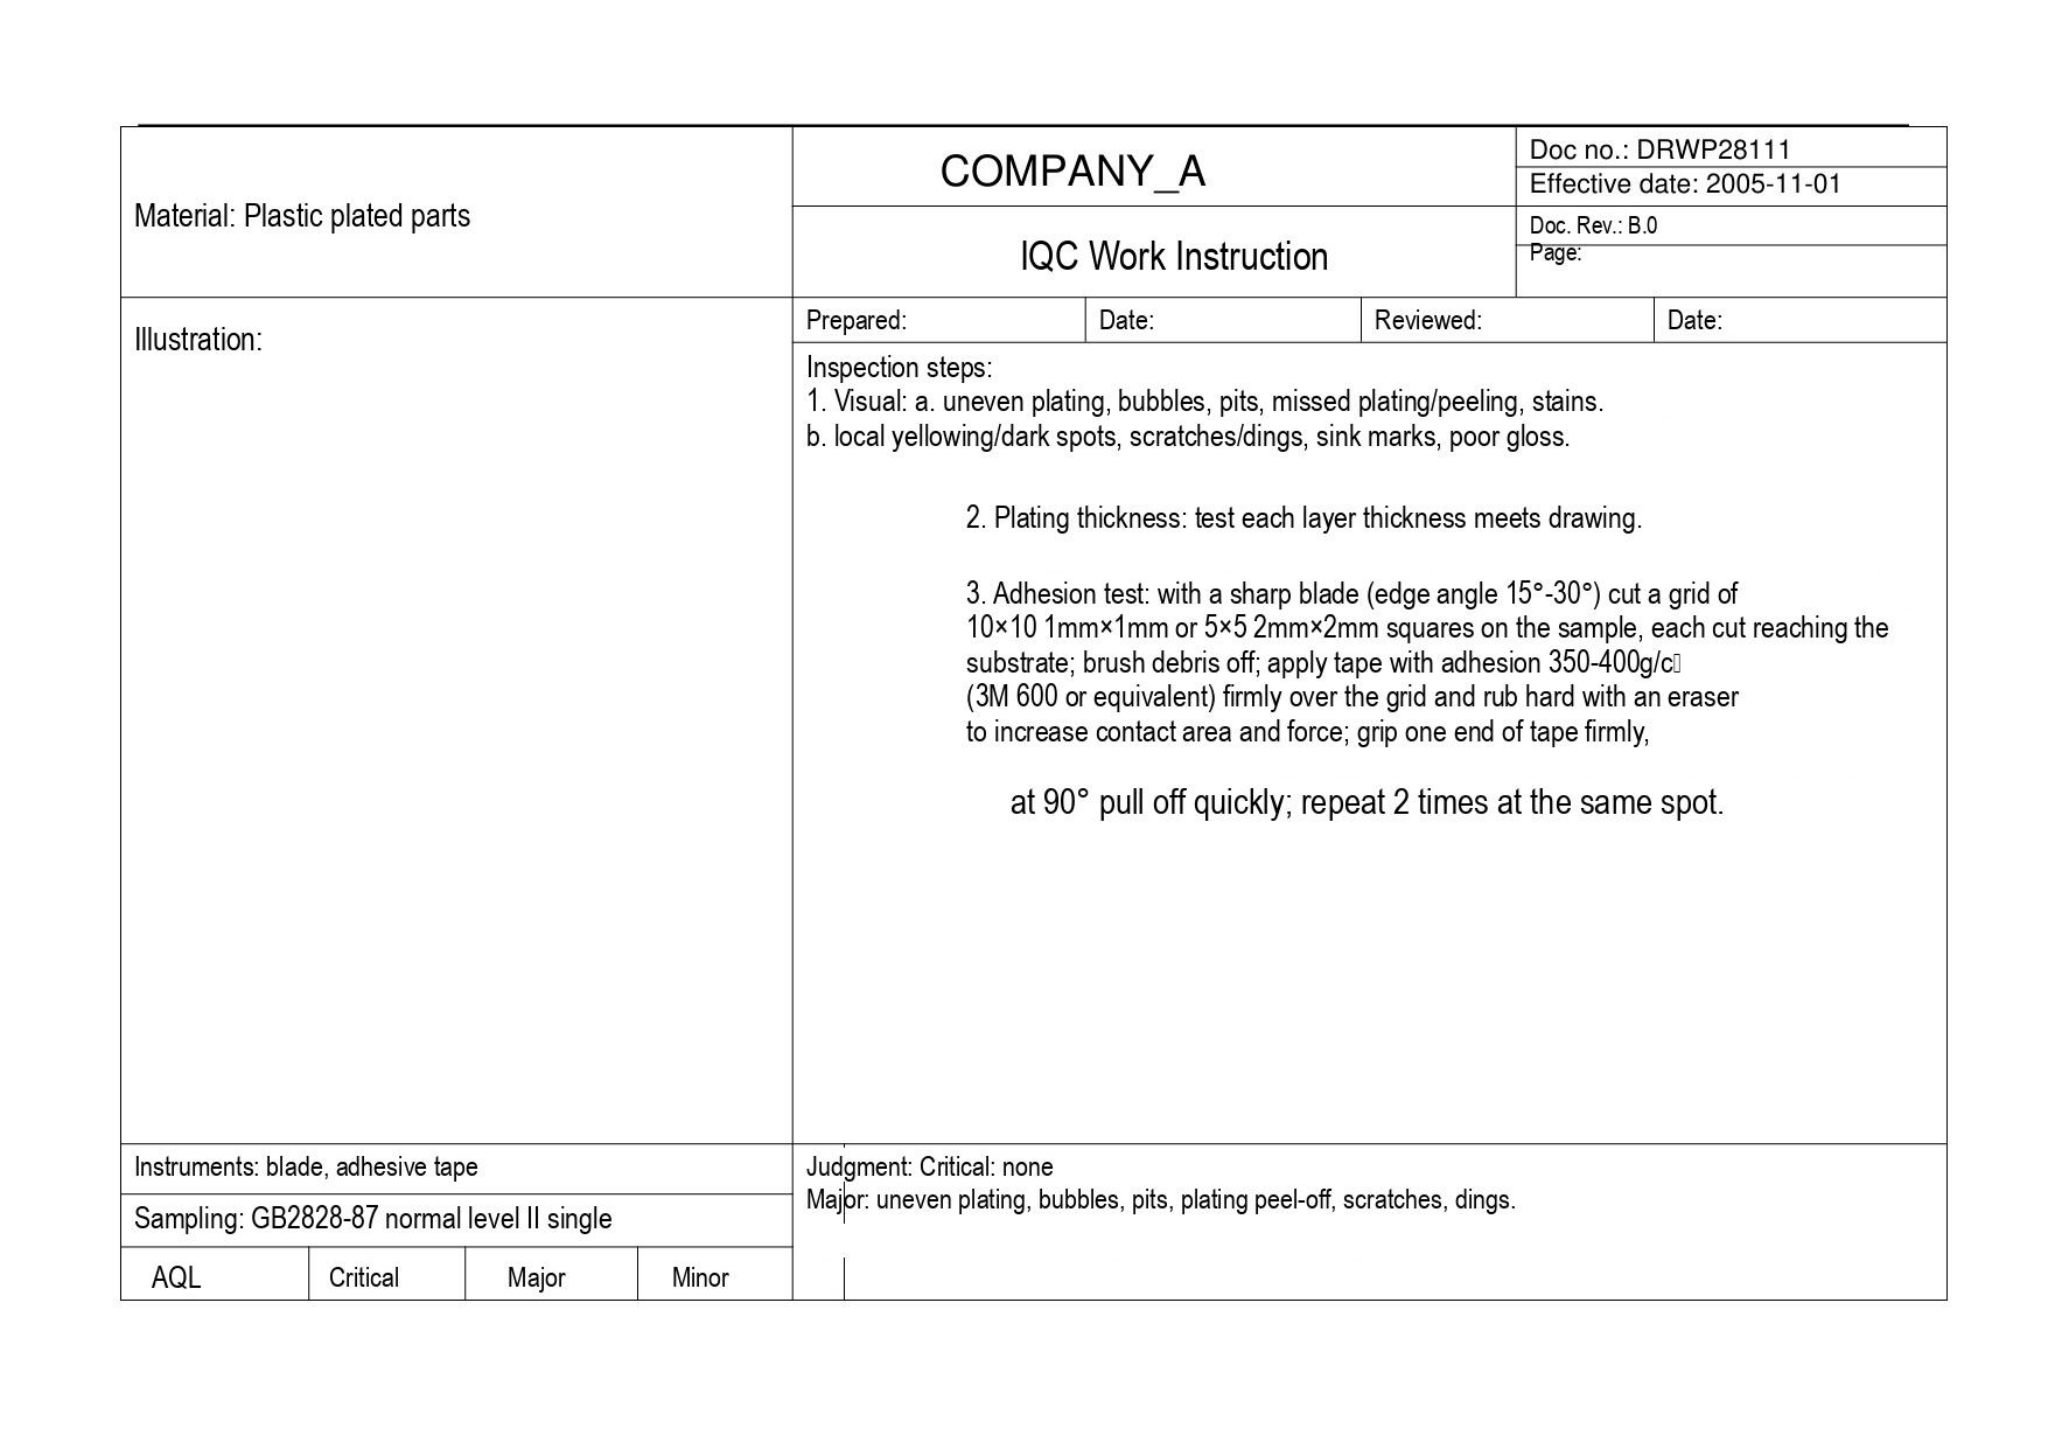| Material: Plastic plated parts | COMPANY_A | Doc no.: DRWP28111 |
|---|---|---|
| | | Effective date: 2005-11-01 |
| | IQC Work Instruction | Doc. Rev.: B.0 |
| | | Page: |

| Prepared: | Date: | Reviewed: | Date: |
|---|---|---|---|

Illustration:

Inspection steps:
1. Visual: a. uneven plating, bubbles, pits, missed plating/peeling, stains.
b. local yellowing/dark spots, scratches/dings, sink marks, poor gloss.

2. Plating thickness: test each layer thickness meets drawing.

3. Adhesion test: with a sharp blade (edge angle 15°-30°) cut a grid of 10×10 1mm×1mm or 5×5 2mm×2mm squares on the sample, each cut reaching the substrate; brush debris off; apply tape with adhesion 350-400g/c
(3M 600 or equivalent) firmly over the grid and rub hard with an eraser to increase contact area and force; grip one end of tape firmly,

at 90° pull off quickly; repeat 2 times at the same spot.

Instruments: blade, adhesive tape

Sampling: GB2828-87 normal level II single

| AQL | Critical | Major | Minor |
|---|---|---|---|

Judgment: Critical: none
Major: uneven plating, bubbles, pits, plating peel-off, scratches, dings.
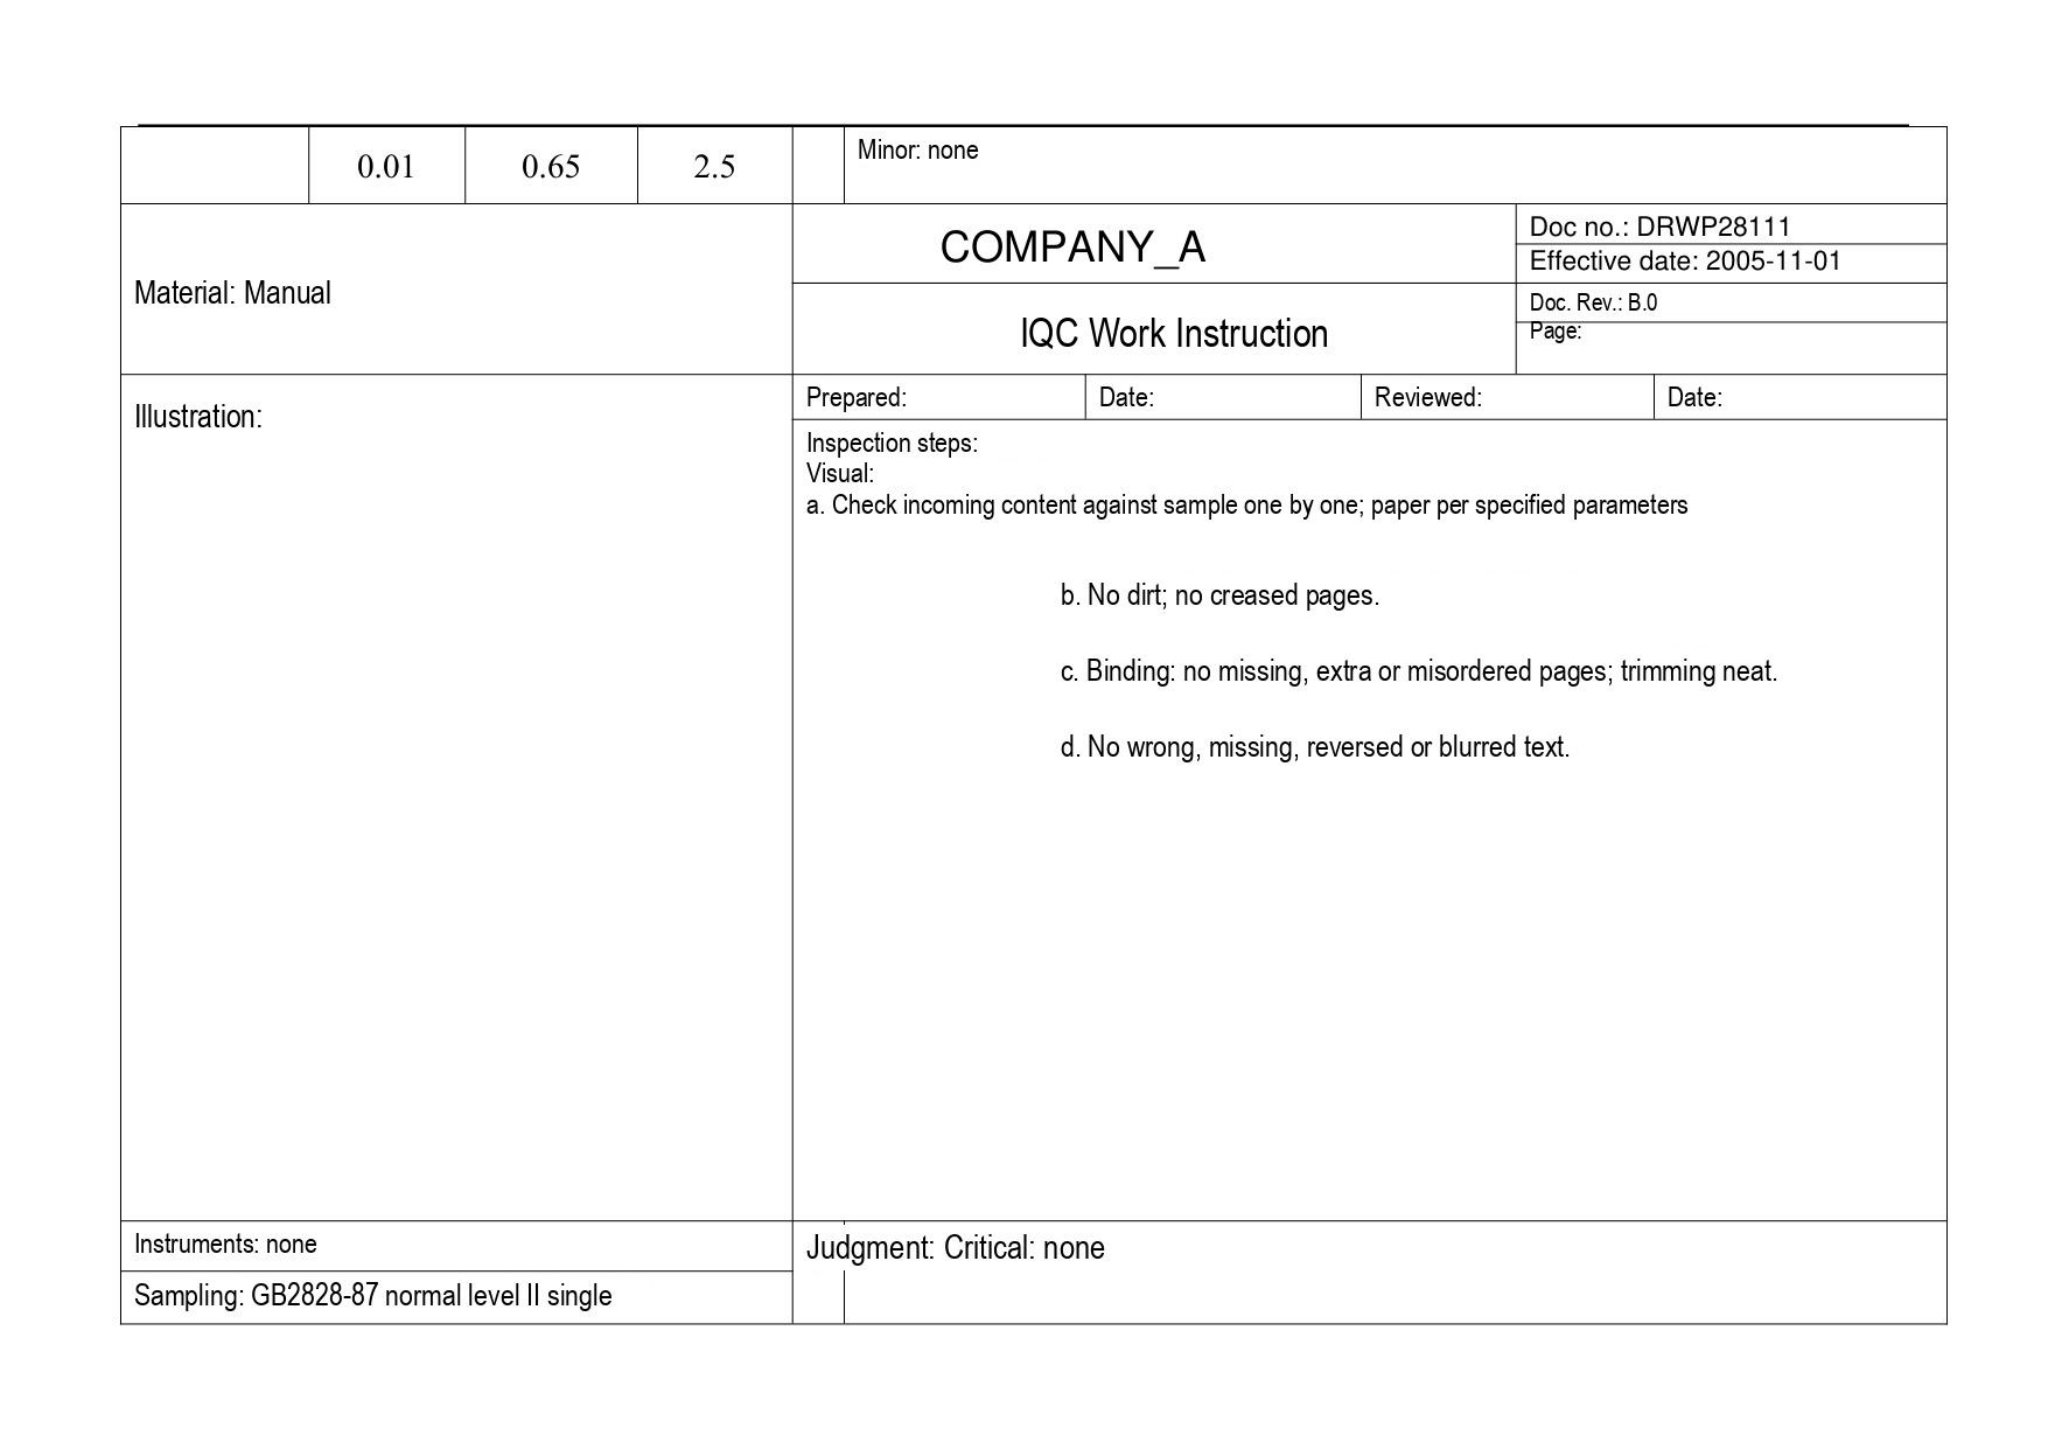| | 0.01 | 0.65 | 2.5 | | Minor: none |
|---|---|---|---|---|---|

Material: Manual

COMPANY_A

IQC Work Instruction

| Doc no.: DRWP28111 |
|---|
| Effective date: 2005-11-01 |
| Doc. Rev.: B.0 |
| Page: |

Illustration:

| Prepared: | Date: | Reviewed: | Date: |
|---|---|---|---|

Inspection steps:
Visual:
a. Check incoming content against sample one by one; paper per specified parameters

b. No dirt; no creased pages.

c. Binding: no missing, extra or misordered pages; trimming neat.

d. No wrong, missing, reversed or blurred text.

Instruments: none

Sampling: GB2828-87 normal level II single

Judgment: Critical: none
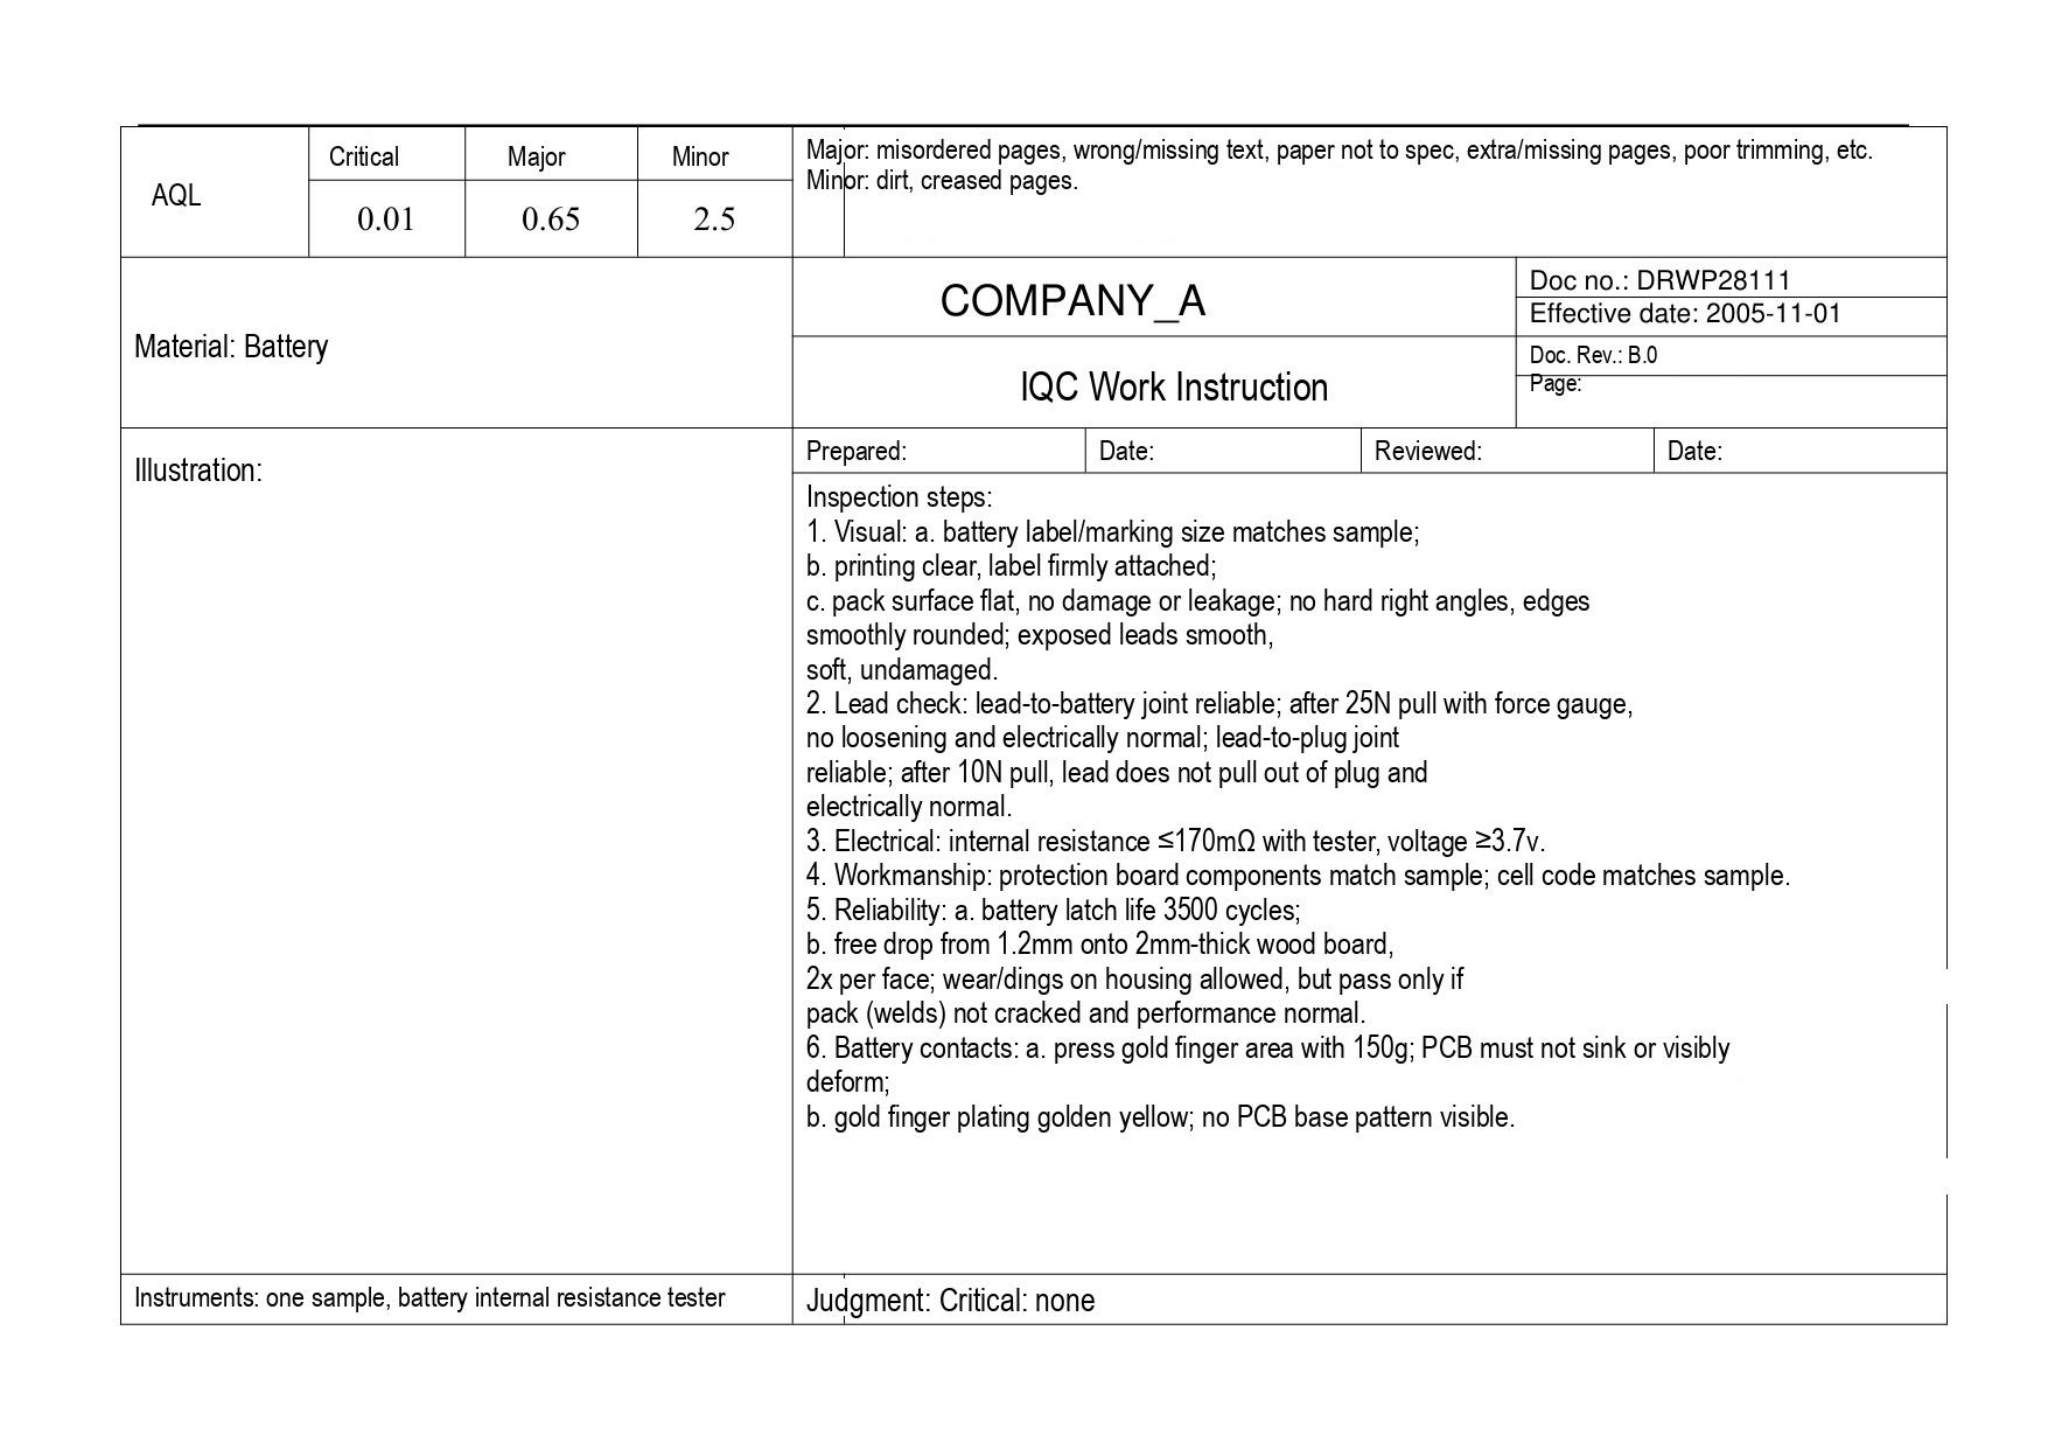| AQL | Critical | Major | Minor |
|---|---|---|---|
| | 0.01 | 0.65 | 2.5 |

Major: misordered pages, wrong/missing text, paper not to spec, extra/missing pages, poor trimming, etc.
Minor: dirt, creased pages.

| Material: Battery | COMPANY_A | Doc no.: DRWP28111 |
|---|---|---|
| | | Effective date: 2005-11-01 |
| | IQC Work Instruction | Doc. Rev.: B.0 |
| | | Page: |

| Prepared: | Date: | Reviewed: | Date: |
|---|---|---|---|

Illustration:

Inspection steps:
1. Visual: a. battery label/marking size matches sample;
b. printing clear, label firmly attached;
c. pack surface flat, no damage or leakage; no hard right angles, edges smoothly rounded; exposed leads smooth, soft, undamaged.
2. Lead check: lead-to-battery joint reliable; after 25N pull with force gauge, no loosening and electrically normal; lead-to-plug joint reliable; after 10N pull, lead does not pull out of plug and electrically normal.
3. Electrical: internal resistance ≤170mΩ with tester, voltage ≥3.7v.
4. Workmanship: protection board components match sample; cell code matches sample.
5. Reliability: a. battery latch life 3500 cycles;
b. free drop from 1.2mm onto 2mm-thick wood board, 2x per face; wear/dings on housing allowed, but pass only if pack (welds) not cracked and performance normal.
6. Battery contacts: a. press gold finger area with 150g; PCB must not sink or visibly deform;
b. gold finger plating golden yellow; no PCB base pattern visible.

| Instruments: one sample, battery internal resistance tester | Judgment: Critical: none |
|---|---|
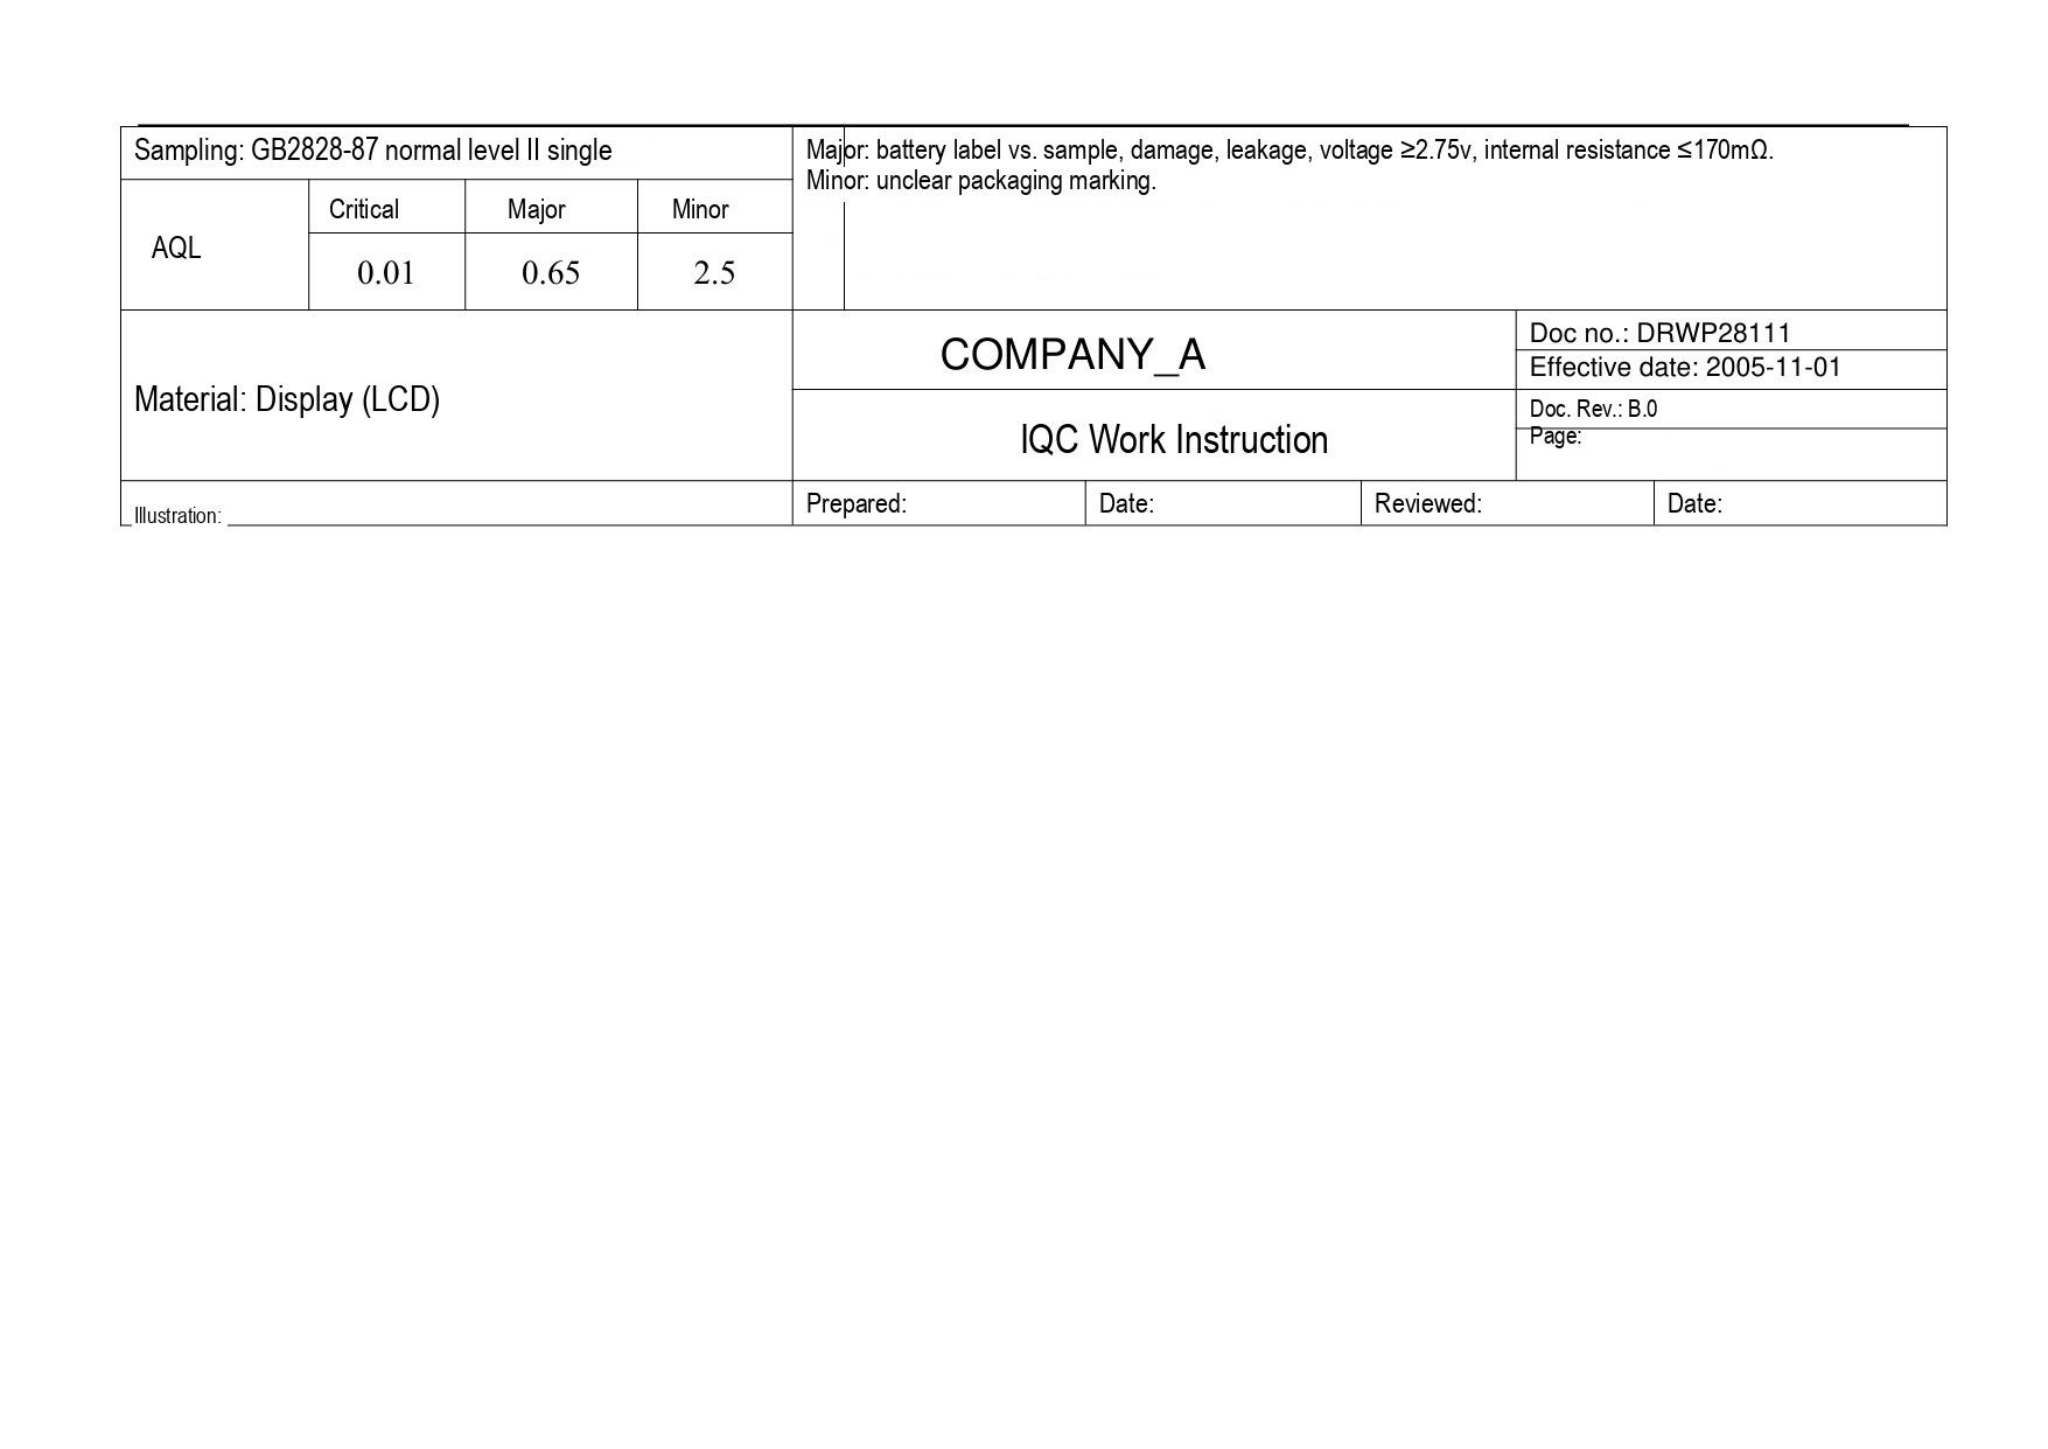| Sampling: GB2828-87 normal level II single | | | | Major: battery label vs. sample, damage, leakage, voltage ≥2.75v, internal resistance ≤170mΩ.<br>Minor: unclear packaging marking. |
|---|---|---|---|---|
| AQL | Critical | Major | Minor | |
| | 0.01 | 0.65 | 2.5 | |

| Material: Display (LCD) | COMPANY_A | Doc no.: DRWP28111<br>Effective date: 2005-11-01 |
|---|---|---|
| | IQC Work Instruction | Doc. Rev.: B.0<br>Page: |

| Illustration: | Prepared: | Date: | Reviewed: | Date: |
|---|---|---|---|---|
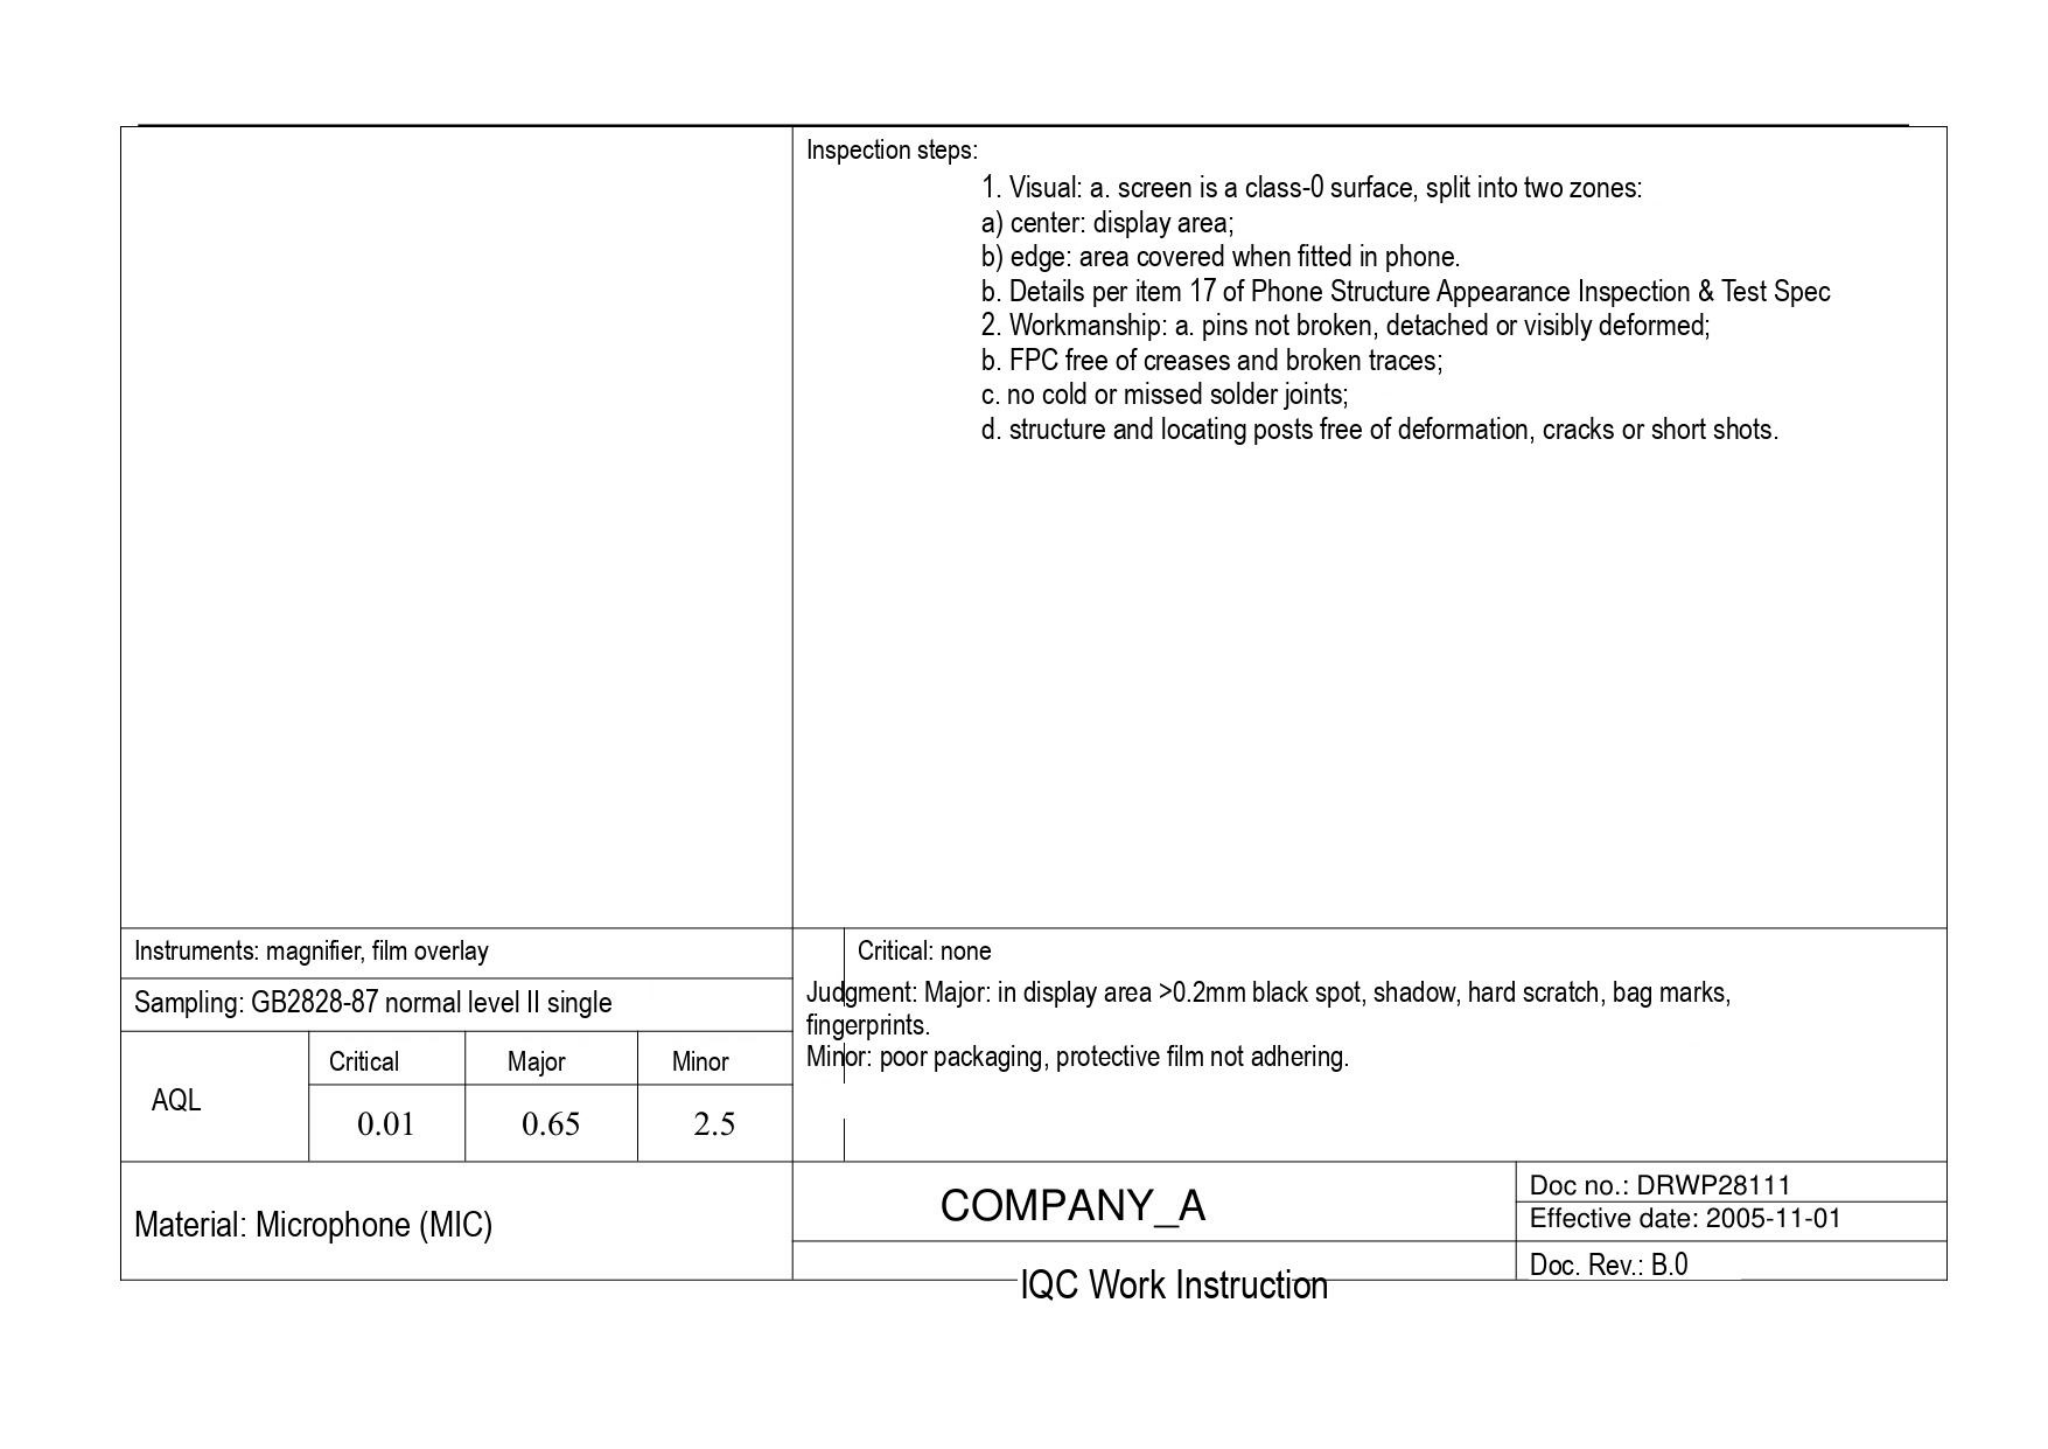Inspection steps:

1. Visual: a. screen is a class-0 surface, split into two zones:
a) center: display area;
b) edge: area covered when fitted in phone.
b. Details per item 17 of Phone Structure Appearance Inspection & Test Spec
2. Workmanship: a. pins not broken, detached or visibly deformed;
b. FPC free of creases and broken traces;
c. no cold or missed solder joints;
d. structure and locating posts free of deformation, cracks or short shots.

Instruments: magnifier, film overlay

Sampling: GB2828-87 normal level II single

| AQL | Critical | Major | Minor |
|---|---|---|---|
| | 0.01 | 0.65 | 2.5 |

Critical: none
Judgment: Major: in display area >0.2mm black spot, shadow, hard scratch, bag marks, fingerprints.
Minor: poor packaging, protective film not adhering.

| Material: Microphone (MIC) | COMPANY_A | Doc no.: DRWP28111 |
|---|---|---|
| | | Effective date: 2005-11-01 |
| | IQC Work Instruction | Doc. Rev.: B.0 |
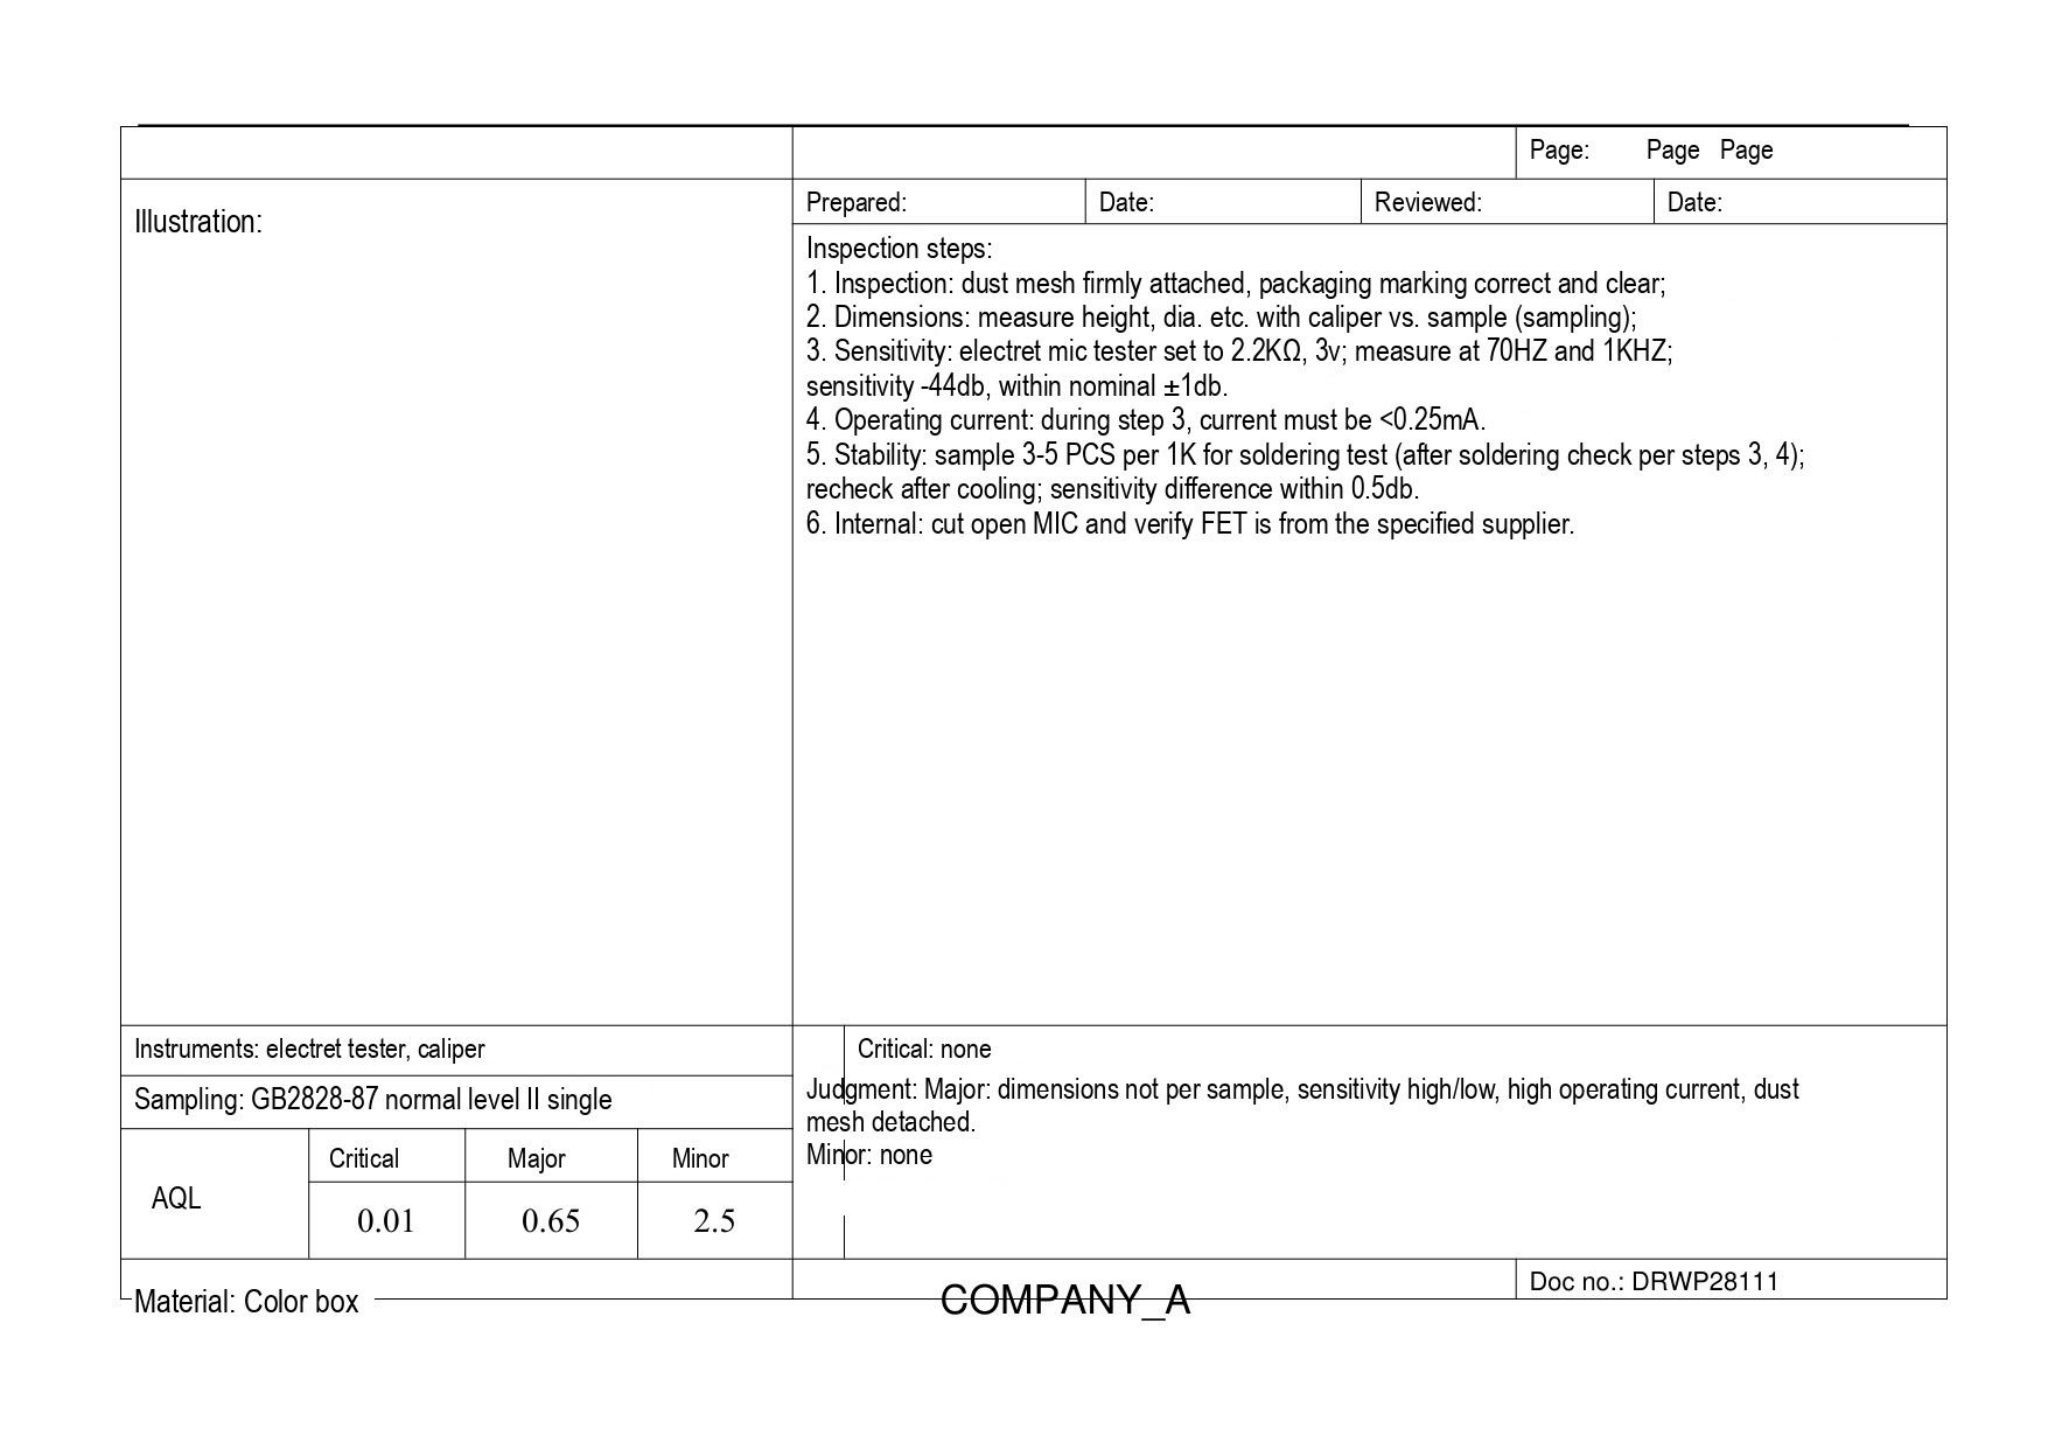Page: Page Page

Illustration:

| Prepared: | Date: | Reviewed: | Date: |
|---|---|---|---|

Inspection steps:
1. Inspection: dust mesh firmly attached, packaging marking correct and clear;
2. Dimensions: measure height, dia. etc. with caliper vs. sample (sampling);
3. Sensitivity: electret mic tester set to 2.2KΩ, 3v; measure at 70HZ and 1KHZ; sensitivity -44db, within nominal ±1db.
4. Operating current: during step 3, current must be <0.25mA.
5. Stability: sample 3-5 PCS per 1K for soldering test (after soldering check per steps 3, 4); recheck after cooling; sensitivity difference within 0.5db.
6. Internal: cut open MIC and verify FET is from the specified supplier.

Instruments: electret tester, caliper

Sampling: GB2828-87 normal level II single

| AQL | Critical | Major | Minor |
|---|---|---|---|
| | 0.01 | 0.65 | 2.5 |

Critical: none
Judgment: Major: dimensions not per sample, sensitivity high/low, high operating current, dust mesh detached.
Minor: none

Material: Color box

COMPANY_A

Doc no.: DRWP28111
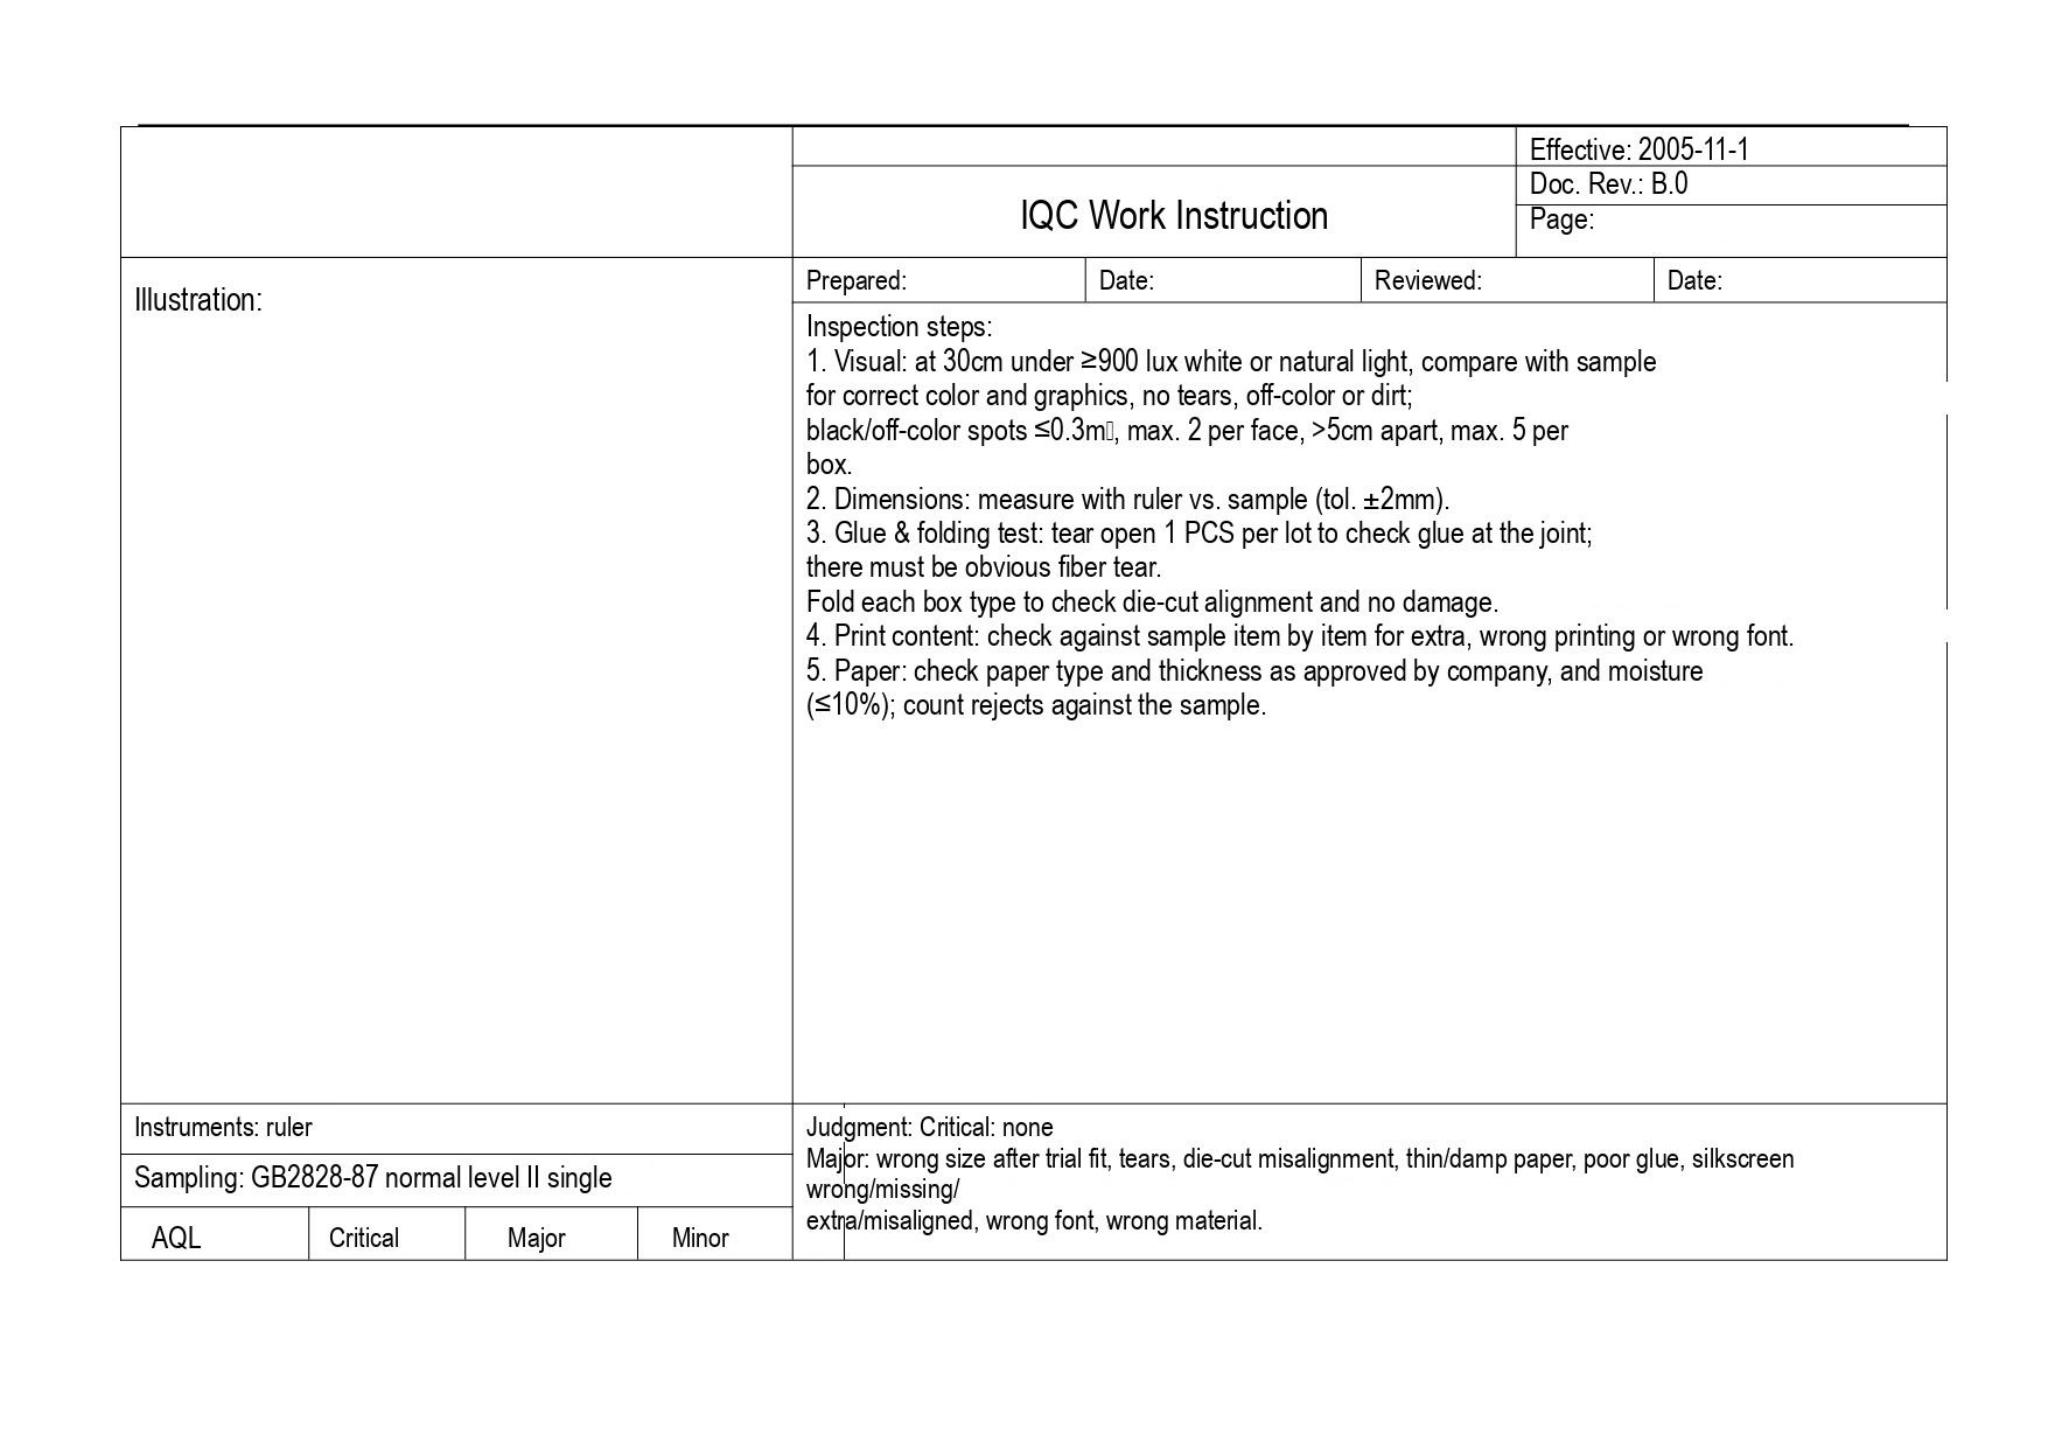| | IQC Work Instruction | Effective: 2005-11-1 |
|---|---|---|
| | | Doc. Rev.: B.0 |
| | | Page: |

| Prepared: | Date: | Reviewed: | Date: |
|---|---|---|---|

Illustration:

Inspection steps:
1. Visual: at 30cm under ≥900 lux white or natural light, compare with sample for correct color and graphics, no tears, off-color or dirt; black/off-color spots ≤0.3m, max. 2 per face, >5cm apart, max. 5 per box.
2. Dimensions: measure with ruler vs. sample (tol. ±2mm).
3. Glue & folding test: tear open 1 PCS per lot to check glue at the joint; there must be obvious fiber tear.
Fold each box type to check die-cut alignment and no damage.
4. Print content: check against sample item by item for extra, wrong printing or wrong font.
5. Paper: check paper type and thickness as approved by company, and moisture (≤10%); count rejects against the sample.

Instruments: ruler

Sampling: GB2828-87 normal level II single

| AQL | Critical | Major | Minor |
|---|---|---|---|

Judgment: Critical: none
Major: wrong size after trial fit, tears, die-cut misalignment, thin/damp paper, poor glue, silkscreen wrong/missing/
extra/misaligned, wrong font, wrong material.